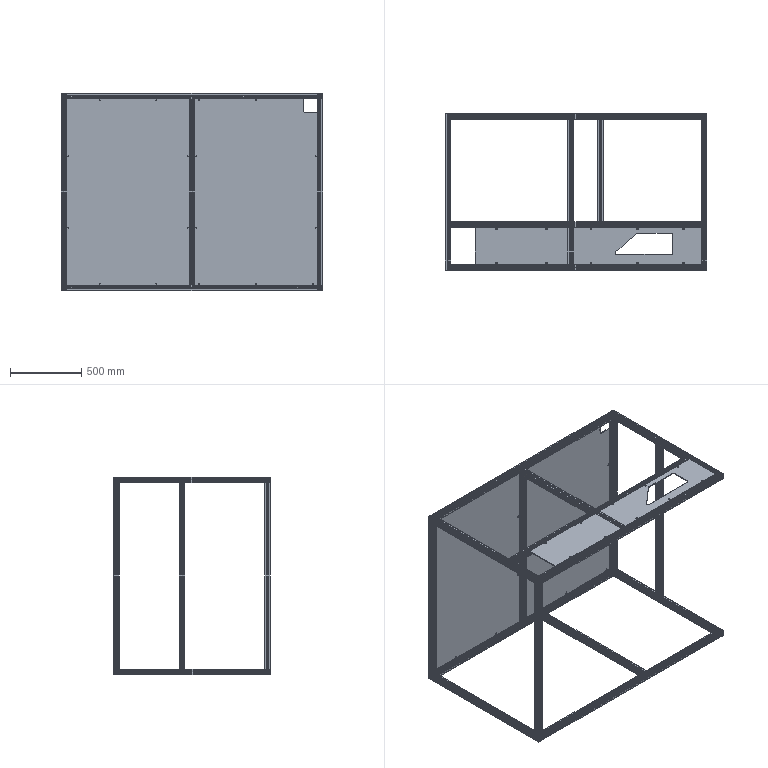Part | SolidWorks | features ICE 16, WeldCornerFeat 14, HoleWzd 8, WeldMemberFeat 7, MirrorPattern 3, Fillet 2, 3DProfileFeature 1, Cut 1, WeldmentFeature 1 | 21 solids | 1398 faces | box 1840 x 1100 x 1390 mm | volume 30476002 mm3 | plane 946 | cylinder 398 | cone 54 | commonest cylinder face diameters 19 x133 8 x112 6.6 x54 6.8 x40 13.3 x17 9 x15